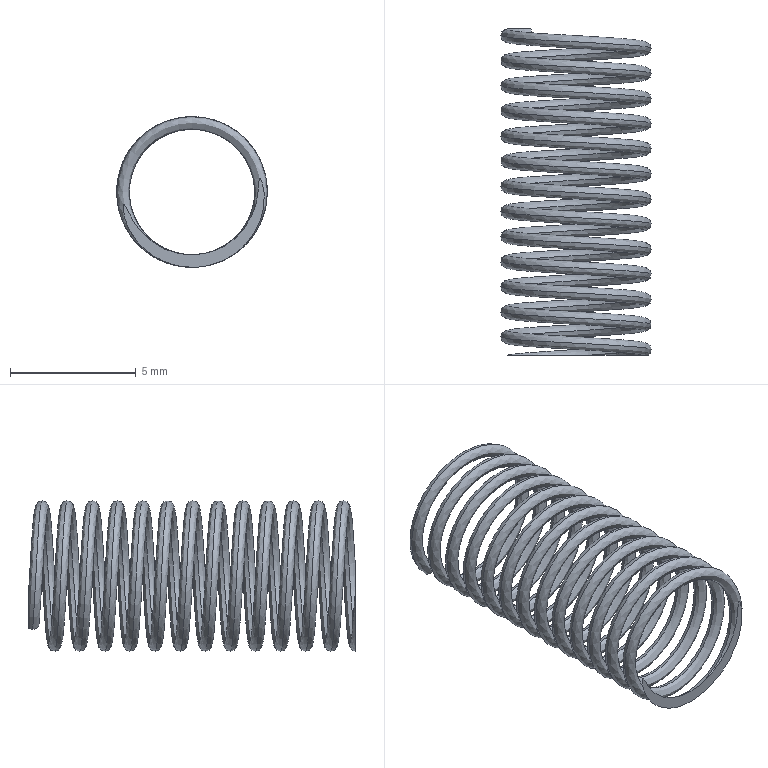Part | SolidWorks | features Helix 1, ICE 1, Sweep 1 | 1 solid | 5 faces | box 6 x 13 x 6 mm | volume 43.094 mm3 | plane 3 | spline 2